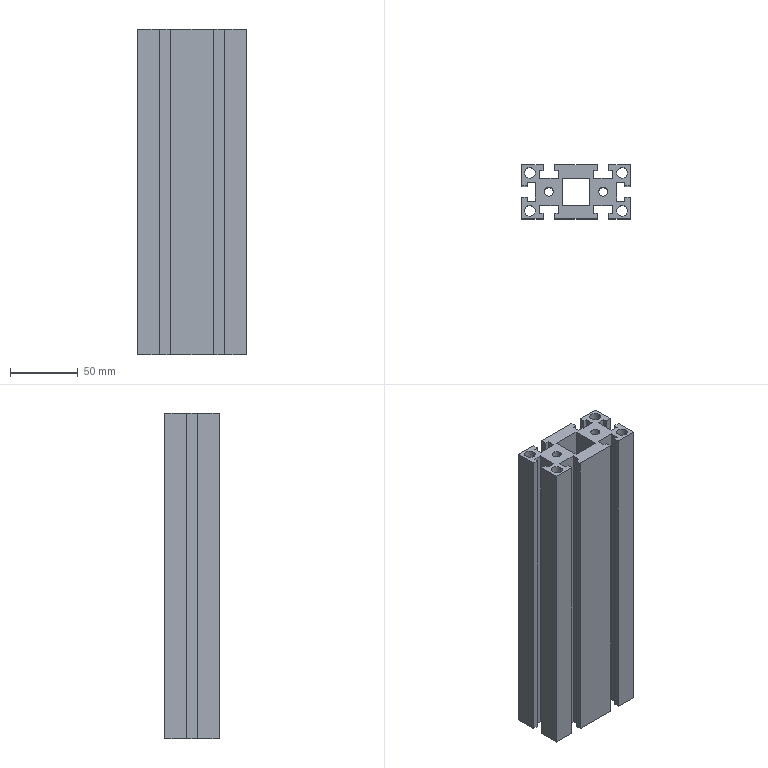Part | STEP file | 1 solid | 70 faces | box 80 x 40 x 240 mm | volume 436902 mm3 | plane 58 | cylinder 12 | commonest cylinder face diameters 8 x8 6.7 x4